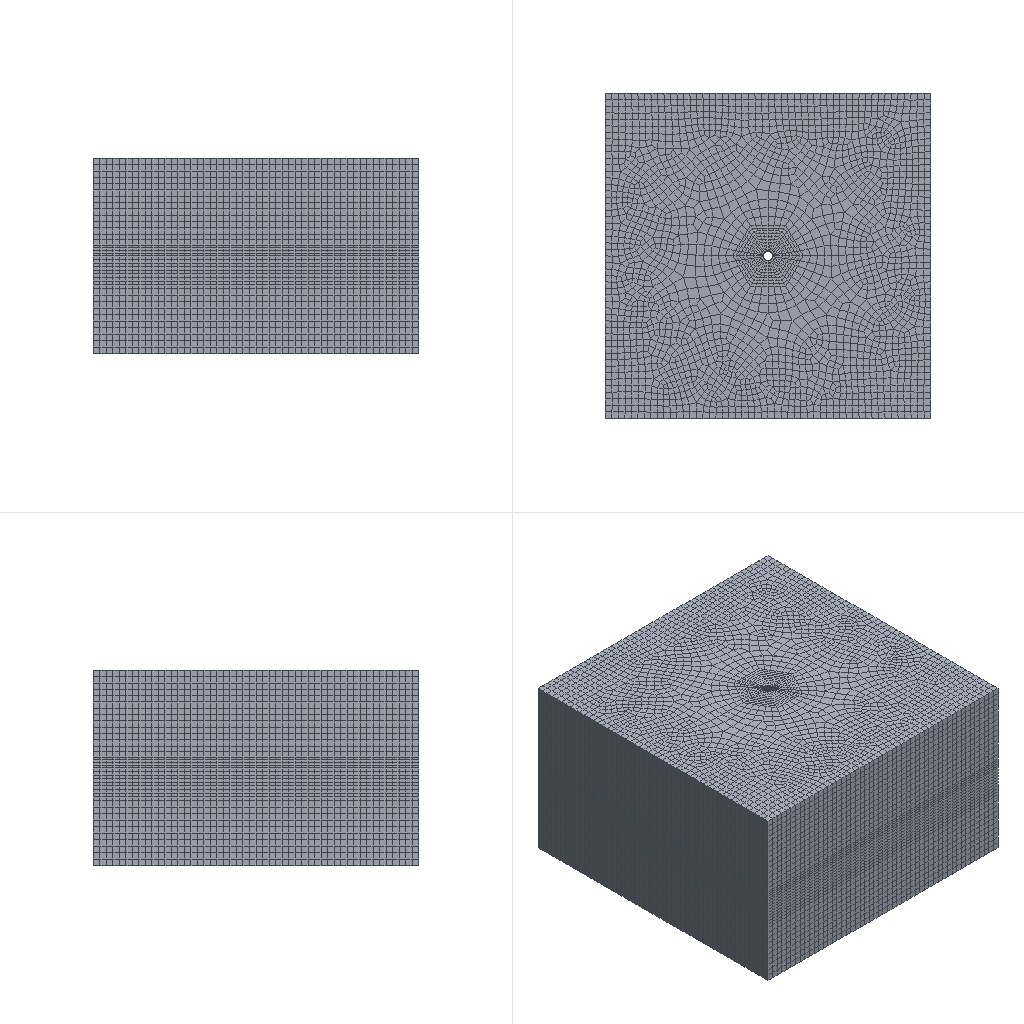Simulation study | abaqus
Set-up summary:
category,name,step,type,value,unit,region
solver,abaqus
solver,version,,,Abaqus/Standard 2020
units,not stated in the deck,,not stated
analysis,deck,,geostatic,geostatic; soils
load_step,Step-1,Step-1,geostatic,nlgeom=False
load_step,Step-2,Step-2,soils,nlgeom=True
contact,interactions,,,general=0 pairs=0 ties=35
load_step,requested,,,2
mesh,nodes,,,104434
mesh,elements,,,96925
element_type,C3D8RP,,solid,96925
load,load commands in deck,,count,3
bc,support commands in deck,,count,6
material,SHUINIHUAN,,in results
material,TAOGUAN,,in results
material,Y,,in results
check,setup vs results,,match,"per instance, exact: element labels, types and connectivity; labels of the nodes the elements use; coordinates of those nodes at SINGLE_PRECISION in 1 of 1 instance(s)"
Abaqus input file, long lists of numbers shortened:
*Heading
** Job name: Job-1 Model name: Model-1-Copy
** Generated by: Abaqus/CAE 2020
*Preprint, echo=NO, model=NO, history=NO, contact=NO
**
** PARTS
**
*Part, name=new
*Node
      1, 0.04, 0.06928,           1.
      2, 0.04, 0.06928,    1.171
** (104432 more lines like these left out)
*Element, type=C3D8RP
 1,   487,     1,   493,  5500,  5503,   502,  5534, 36186
 2,  5501,   490,   489,  5499, 36187,  5518,  5519, 36185
** (96923 more lines like these left out)
*Nset, nset=Set-40
     1,     2,     3,     4,     5,    11,    14,    15,    18,    19,    22,    23,    26,    27,    30,    46
    47,    48,    49,    50,    51,    52,    53,    54,    55,    56,    65,    66,    67,    68,    69,    70
** (166 more lines like these left out)
*Elset, elset=Set-40
   964,   965,   966,   967,   968,   969,   970,   971,   972,   973,   974,   975,   976,   977,   978,   979
   980,   981,   982,   983,   984,   985,   986,   987,   988,   989,   990,   991,   992,   993,   994,   995
** (79 more lines like these left out)
*Nset, nset=Set-41
     1,     2,     3,     4,     5,    11,    14,    15,    18,    19,    22,    23,    26,    27,    30,    46
    47,    48,    49,    50,    51,    52,    53,    54,    55,    56,    65,    66,    67,    68,    69,    70
** (166 more lines like these left out)
*Elset, elset=Set-41
   964,   965,   966,   967,   968,   969,   970,   971,   972,   973,   974,   975,   976,   977,   978,   979
   980,   981,   982,   983,   984,   985,   986,   987,   988,   989,   990,   991,   992,   993,   994,   995
** (79 more lines like these left out)
*Nset, nset=Set-42, generate
      1,  104434,       1
*Elset, elset=Set-42, generate
     1,  96925,      1
** Section: Section-2
*Solid Section, elset=Set-42, material=shuinihuan
,
*End Part
**
**
** ASSEMBLY
**
*Assembly, name=Assembly
**
*Instance, name=new-1, part=new
*End Instance
**
*Nset, nset=Set-5, instance=new-1
     9,    10,    31,    49,    55,    58,    62,    63,    68,    69,    75,    76,    77,    83,    84,    88
    90,    91,    97,   102,   104,   105,   108,   133,   144,   166,   178,   179,   182,   189,   190,   191
** (6 more lines like these left out)
*Elset, elset=Set-5, instance=new-1
   729,  1269,  1413,  1415,  1488,  1517,  1518,  1523,  1542,  1753,  1834,  2053,  2133,  2138,  2152,  2478
  2479,  2480,  2481,  3579,  3580,  3584,  3587,  3711,  4756,  5511,  6123,  6259,  6263,  6270,  6273,  6971
** (3 more lines like these left out)
*Nset, nset=Set-6, instance=new-1
     9,    10,    31,    49,    55,    58,    62,    63,    68,    69,    75,    76,    77,    83,    84,    88
    90,    91,    97,   102,   104,   105,   108,   133,   144,   166,   178,   179,   182,   189,   190,   191
** (6 more lines like these left out)
*Elset, elset=Set-6, instance=new-1
   729,  1269,  1413,  1415,  1488,  1517,  1518,  1523,  1542,  1753,  1834,  2053,  2133,  2138,  2152,  2478
  2479,  2480,  2481,  3579,  3580,  3584,  3587,  3711,  4756,  5511,  6123,  6259,  6263,  6270,  6273,  6971
** (3 more lines like these left out)
*Nset, nset=Set-7, instance=new-1
   426,   427,   428,   429,   430,   431,   432,   433,   434,   435,   436,   437,   438,   439,   440,   441
   447,   448,   449,   450,   456,   457,   458,   459,   479,   480,   481,   482,   483,   484,   485,   486
** (241 more lines like these left out)
*Elset, elset=Set-7, instance=new-1
 15663, 15666, 15667, 15668, 15690, 15691, 15692, 15694, 15695, 15696, 15746, 15747, 15749, 15772, 15774, 15804
 15805, 15808, 15810, 15822, 15834, 15835, 15836, 15845, 15850, 15852, 15859, 15860, 15861, 15863, 15865, 15866
** (230 more lines like these left out)
*Nset, nset=Set-8, instance=new-1
   426,   427,   428,   429,   430,   431,   432,   433,   434,   435,   436,   437,   438,   439,   440,   441
   447,   448,   449,   450,   456,   457,   458,   459,   479,   480,   481,   482,   483,   484,   485,   486
** (241 more lines like these left out)
*Elset, elset=Set-8, instance=new-1
 15663, 15669, 15713, 15714, 15716, 15717, 15718, 15720, 15731, 15787, 15788, 15790, 15792, 15811, 15823, 15824
 15826, 15827, 15828, 15840, 15841, 15847, 15848, 15850, 15920, 15922, 15924, 15925, 15927, 15929, 15930, 15932
** (230 more lines like these left out)
*Nset, nset=Set-9, instance=new-1
    27,    28,    29,    30,    44,    45,    51,    53,    54,    56,    57,    59,    60,    61,    85,    87
    89,    93,    96,    98,    99,   100,   101,   121,   122,   123,   124,   139,   140,   141,   142,   152
** (342 more lines like these left out)
*Elset, elset=Set-9, instance=new-1
   694,   695,   696,   697,   698,   699,   700,   701,   702,   703,   704,   705,   706,   707,   708,   709
   710,   711,   712,   713,   714,   715,   716,   717,   718,   719,   720,   955,   956,   957,   958,   959
** (335 more lines like these left out)
*Nset, nset=Set-10, instance=new-1
   426,   427,   428,   429,   430,   431,   432,   433,   434,   435,   436,   437,   438,   439,   440,   441
   447,   448,   449,   450,   456,   457,   458,   459,   479,   480,   481,   482,   483,   484,   485,   486
** (473 more lines like these left out)
*Elset, elset=Set-10, instance=new-1
 15663, 15666, 15667, 15668, 15669, 15690, 15691, 15692, 15694, 15695, 15696, 15713, 15714, 15716, 15717, 15718
 15720, 15731, 15746, 15747, 15749, 15772, 15774, 15787, 15788, 15790, 15792, 15804, 15805, 15808, 15810, 15811
** (452 more lines like these left out)
*Nset, nset=Set-11, instance=new-1
     3,     4,     5,     8,     9,    10,    13,    14,    17,    18,    21,    22,    25,    26,    29,    30
    46,    47,    48,    49,    50,    52,    53,    54,    55,    56,    58,    59,    62,    63,    64,    65
** (244 more lines like these left out)
*Elset, elset=Set-11, instance=new-1
     3,     5,     6,     8,    11,    13,    14,    16,    19,    21,    22,    24,    27,    29,    30,    32
    35,    37,    38,    40,    43,    45,    46,    48,    51,    53,    54,    56,    59,    61,    62,    64
** (339 more lines like these left out)
*Nset, nset=Set-12, instance=new-1, generate
      1,  104434,       1
*Elset, elset=Set-12, instance=new-1, generate
     1,  96925,      1
*Nset, nset=Set-13, instance=new-1, generate
      1,  104434,       1
*Elset, elset=Set-13, instance=new-1, generate
     1,  96925,      1
*Nset, nset=Set-14, instance=new-1, generate
      1,  104434,       1
*Elset, elset=Set-14, instance=new-1, generate
     1,  96925,      1
*Elset, elset=__T0_new-1_M_S2, internal, instance=new-1, generate
 739,  747,    1
*Surface, type=ELEMENT, name=_T0_new-1_M, internal
__T0_new-1_M_S2, S2
*Elset, elset=__T0_new-1_S_S3, internal, instance=new-1
 71304,
*Surface, type=ELEMENT, name=_T0_new-1_S, internal
__T0_new-1_S_S3, S3
*Tie, name=_T0_new-1, adjust=no
_T0_new-1_S, _T0_new-1_M
*Elset, elset=__T1_new-1_M_S2, internal, instance=new-1, generate
 1298,  1325,     1
*Surface, type=ELEMENT, name=_T1_new-1_M, internal
__T1_new-1_M_S2, S2
*Elset, elset=__T1_new-1_S_S3, internal, instance=new-1, generate
 77799,  92954,   2165
*Surface, type=ELEMENT, name=_T1_new-1_S, internal
__T1_new-1_S_S3, S3
*Tie, name=_T1_new-1, adjust=no
_T1_new-1_S, _T1_new-1_M
*Elset, elset=__T2_new-1_M_S4, internal, instance=new-1
 42011, 44176
*Elset, elset=__T2_new-1_M_S6, internal, instance=new-1
 42010, 44175
*Elset, elset=__T2_new-1_M_S5, internal, instance=new-1
 42009, 44174
*Surface, type=ELEMENT, name=_T2_new-1_M, internal
__T2_new-1_M_S4, S4
__T2_new-1_M_S6, S6
__T2_new-1_M_S5, S5
*Elset, elset=__T2_new-1_S_S2, internal, instance=new-1
 1511,
*Surface, type=ELEMENT, name=_T2_new-1_S, internal
__T2_new-1_S_S2, S2
*Tie, name=_T2_new-1, adjust=no
_T2_new-1_S, _T2_new-1_M
*Nset, nset=_T2_new-1_SN, instance=new-1
 6563,
*Surface, type=NODE, name=_T2_new-1_SN, internal
_T2_new-1_SN
*Tie, name=_T2_new-1-Nodes, adjust=no
_T2_new-1_SN, _T2_new-1_M
*Elset, elset=__T3_new-1_M_S2, internal, instance=new-1, generate
 1801,  1824,     1
*Surface, type=ELEMENT, name=_T3_new-1_M, internal
__T3_new-1_M_S2, S2
*Elset, elset=__T3_new-1_S_S6, internal, instance=new-1, generate
 77808,  92963,   2165
*Surface, type=ELEMENT, name=_T3_new-1_S, internal
__T3_new-1_S_S6, S6
*Tie, name=_T3_new-1, adjust=no
_T3_new-1_S, _T3_new-1_M
*Elset, elset=__T4_new-1_M_S4, internal, instance=new-1, generate
 69149,  73479,   2165
*Elset, elset=__T4_new-1_M_S6, internal, instance=new-1, generate
 69148,  73478,   2165
*Elset, elset=__T4_new-1_M_S5, internal, instance=new-1, generate
 69147,  73477,   2165
*Surface, type=ELEMENT, name=_T4_new-1_M, internal
__T4_new-1_M_S4, S4
__T4_new-1_M_S6, S6
__T4_new-1_M_S5, S5
*Elset, elset=__T4_new-1_S_S2, internal, instance=new-1
 1849,
*Surface, type=ELEMENT, name=_T4_new-1_S, internal
__T4_new-1_S_S2, S2
*Tie, name=_T4_new-1, adjust=no
_T4_new-1_S, _T4_new-1_M
*Nset, nset=_T4_new-1_SN, instance=new-1
 6759,
*Surface, type=NODE, name=_T4_new-1_SN, internal
_T4_new-1_SN
*Tie, name=_T4_new-1-Nodes, adjust=no
_T4_new-1_SN, _T4_new-1_M
*Elset, elset=__T5_new-1_M_S2, internal, instance=new-1, generate
 2099,  2121,     1
*Surface, type=ELEMENT, name=_T5_new-1_M, internal
__T5_new-1_M_S2, S2
*Elset, elset=__T5_new-1_S_S6, internal, instance=new-1, generate
 18195,  37680,   2165
*Surface, type=ELEMENT, name=_T5_new-1_S, internal
__T5_new-1_S_S6, S6
*Tie, name=_T5_new-1, adjust=no
_T5_new-1_S, _T5_new-1_M
*Elset, elset=__T6_new-1_M_S2, internal, instance=new-1, generate
 2162,  2170,     1
*Surface, type=ELEMENT, name=_T6_new-1_M, internal
__T6_new-1_M_S2, S2
*Elset, elset=__T6_new-1_S_S6, internal, instance=new-1
 57506,
*Surface, type=ELEMENT, name=_T6_new-1_S, internal
__T6_new-1_S_S6, S6
*Tie, name=_T6_new-1, adjust=no
_T6_new-1_S, _T6_new-1_M
*Elset, elset=__T7_new-1_M_S5, internal, instance=new-1, generate
 47995,  54490,   2165
*Elset, elset=__T7_new-1_M_S6, internal, instance=new-1, generate
 46369,  52864,   2165
*Elset, elset=__T7_new-1_M_S4, internal, instance=new-1, generate
 46368,  52863,   2165
*Surface, type=ELEMENT, name=_T7_new-1_M, internal
__T7_new-1_M_S5, S5
__T7_new-1_M_S6, S6
__T7_new-1_M_S4, S4
*Elset, elset=__T7_new-1_S_S2, internal, instance=new-1
 2501,
*Surface, type=ELEMENT, name=_T7_new-1_S, internal
__T7_new-1_S_S2, S2
*Tie, name=_T7_new-1, adjust=no
_T7_new-1_S, _T7_new-1_M
*Nset, nset=_T7_new-1_SN, instance=new-1
 7236, 7237, 7241, 7243, 7244
*Surface, type=NODE, name=_T7_new-1_SN, internal
_T7_new-1_SN
*Tie, name=_T7_new-1-Nodes, adjust=no
_T7_new-1_SN, _T7_new-1_M
*Elset, elset=__T8_new-1_M_S2, internal, instance=new-1, generate
 3721,  3729,     1
*Surface, type=ELEMENT, name=_T8_new-1_M, internal
__T8_new-1_M_S2, S2
*Elset, elset=__T8_new-1_S_S3, internal, instance=new-1
 65862,
*Surface, type=ELEMENT, name=_T8_new-1_S, internal
__T8_new-1_S_S3, S3
*Tie, name=_T8_new-1, adjust=no
_T8_new-1_S, _T8_new-1_M
*Elset, elset=__T9_new-1_M_S2, internal, instance=new-1, generate
 4774,  4782,     1
*Surface, type=ELEMENT, name=_T9_new-1_M, internal
__T9_new-1_M_S2, S2
*Elset, elset=__T9_new-1_S_S3, internal, instance=new-1
 59133,
*Surface, type=ELEMENT, name=_T9_new-1_S, internal
__T9_new-1_S_S3, S3
*Tie, name=_T9_new-1, adjust=no
_T9_new-1_S, _T9_new-1_M
*Elset, elset=__T10_new-1_M_S2, internal, instance=new-1, generate
 5521,  5529,     1
*Surface, type=ELEMENT, name=_T10_new-1_M, internal
__T10_new-1_M_S2, S2
*Elset, elset=__T10_new-1_S_S6, internal, instance=new-1
 57230,
*Surface, type=ELEMENT, name=_T10_new-1_S, internal
__T10_new-1_S_S6, S6
*Tie, name=_T10_new-1, adjust=no
_T10_new-1_S, _T10_new-1_M
*Elset, elset=__T11_new-1_M_S2, internal, instance=new-1, generate
 6133,  6141,     1
*Surface, type=ELEMENT, name=_T11_new-1_M, internal
__T11_new-1_M_S2, S2
*Elset, elset=__T11_new-1_S_S6, internal, instance=new-1
 63959,
*Surface, type=ELEMENT, name=_T11_new-1_S, internal
__T11_new-1_S_S6, S6
*Tie, name=_T11_new-1, adjust=no
_T11_new-1_S, _T11_new-1_M
*Elset, elset=__T12_new-1_M_S5, internal, instance=new-1
 62027, 62398, 64192, 64563, 66357, 66728
*Elset, elset=__T12_new-1_M_S3, internal, instance=new-1, generate
 63739,  68069,   2165
*Surface, type=ELEMENT, name=_T12_new-1_M, internal
__T12_new-1_M_S5, S5
__T12_new-1_M_S3, S3
*Elset, elset=__T12_new-1_S_S2, internal, instance=new-1
 6982,
*Surface, type=ELEMENT, name=_T12_new-1_S, internal
__T12_new-1_S_S2, S2
*Tie, name=_T12_new-1, adjust=no
_T12_new-1_S, _T12_new-1_M
*Nset, nset=_T12_new-1_SN, instance=new-1
 9599,
*Surface, type=NODE, name=_T12_new-1_SN, internal
_T12_new-1_SN
*Tie, name=_T12_new-1-Nodes, adjust=no
_T12_new-1_SN, _T12_new-1_M
*Elset, elset=__T13_new-1_M_S2, internal, instance=new-1, generate
 7541,  7549,     1
*Surface, type=ELEMENT, name=_T13_new-1_M, internal
__T13_new-1_M_S2, S2
*Elset, elset=__T13_new-1_S_S5, internal, instance=new-1
 71299,
*Surface, type=ELEMENT, name=_T13_new-1_S, internal
__T13_new-1_S_S5, S5
*Tie, name=_T13_new-1, adjust=no
_T13_new-1_S, _T13_new-1_M
*Elset, elset=__T14_new-1_M_S6, internal, instance=new-1
 42019, 42025, 44184, 44190
*Elset, elset=__T14_new-1_M_S4, internal, instance=new-1
 43659, 45824
*Surface, type=ELEMENT, name=_T14_new-1_M, internal
__T14_new-1_M_S6, S6
__T14_new-1_M_S4, S4
*Nset, nset=_T14_new-1_SN, instance=new-1, generate
 9948,  9950,     1
*Surface, type=NODE, name=_T14_new-1_SN, internal
_T14_new-1_SN
*Tie, name=_T14_new-1-Nodes, adjust=no
_T14_new-1_SN, _T14_new-1_M
*Elset, elset=__T15_new-1_M_S2, internal, instance=new-1, generate
 7974,  7998,     1
*Surface, type=ELEMENT, name=_T15_new-1_M, internal
__T15_new-1_M_S2, S2
*Elset, elset=__T15_new-1_S_S6, internal, instance=new-1, generate
 18204,  37689,   2165
*Surface, type=ELEMENT, name=_T15_new-1_S, internal
__T15_new-1_S_S6, S6
*Tie, name=_T15_new-1, adjust=no
_T15_new-1_S, _T15_new-1_M
*Elset, elset=__T16_new-1_M_S2, internal, instance=new-1, generate
 8321,  8345,     1
*Surface, type=ELEMENT, name=_T16_new-1_M, internal
__T16_new-1_M_S2, S2
*Elset, elset=__T16_new-1_S_S6, internal, instance=new-1, generate
 77817,  92972,   2165
*Surface, type=ELEMENT, name=_T16_new-1_S, internal
__T16_new-1_S_S6, S6
*Tie, name=_T16_new-1, adjust=no
_T16_new-1_S, _T16_new-1_M
*Elset, elset=__T17_new-1_M_S2, internal, instance=new-1, generate
 8496,  8504,     1
*Surface, type=ELEMENT, name=_T17_new-1_M, internal
__T17_new-1_M_S2, S2
*Elset, elset=__T17_new-1_S_S6, internal, instance=new-1
 71322,
*Surface, type=ELEMENT, name=_T17_new-1_S, internal
__T17_new-1_S_S6, S6
*Tie, name=_T17_new-1, adjust=no
_T17_new-1_S, _T17_new-1_M
*Elset, elset=__T18_new-1_M_S5, internal, instance=new-1
 42027, 43662, 44192, 45827
*Elset, elset=__T18_new-1_M_S4, internal, instance=new-1
 42026, 44191
*Surface, type=ELEMENT, name=_T18_new-1_M, internal
__T18_new-1_M_S5, S5
__T18_new-1_M_S4, S4
*Elset, elset=__T18_new-1_S_S2, internal, instance=new-1
 9031,
*Surface, type=ELEMENT, name=_T18_new-1_S, internal
__T18_new-1_S_S2, S2
*Tie, name=_T18_new-1, adjust=no
_T18_new-1_S, _T18_new-1_M
*Nset, nset=_T18_new-1_SN, instance=new-1
 10750,
*Surface, type=NODE, name=_T18_new-1_SN, internal
_T18_new-1_SN
*Tie, name=_T18_new-1-Nodes, adjust=no
_T18_new-1_SN, _T18_new-1_M
*Elset, elset=__T19_new-1_M_S2, internal, instance=new-1, generate
 9760,  9769,     1
*Surface, type=ELEMENT, name=_T19_new-1_M, internal
__T19_new-1_M_S2, S2
*Elset, elset=__T19_new-1_S_S5, internal, instance=new-1
 48522, 50687
*Surface, type=ELEMENT, name=_T19_new-1_S, internal
__T19_new-1_S_S5, S5
*Tie, name=_T19_new-1, adjust=no
_T19_new-1_S, _T19_new-1_M
*Elset, elset=__T20_new-1_M_S2, internal, instance=new-1, generate
 9959,  9967,     1
*Surface, type=ELEMENT, name=_T20_new-1_M, internal
__T20_new-1_M_S2, S2
*Elset, elset=__T20_new-1_S_S6, internal, instance=new-1
 71297,
*Surface, type=ELEMENT, name=_T20_new-1_S, internal
__T20_new-1_S_S6, S6
*Tie, name=_T20_new-1, adjust=no
_T20_new-1_S, _T20_new-1_M
*Elset, elset=__T21_new-1_M_S6, internal, instance=new-1
 62023, 62025, 64188, 64190, 66353, 66355
*Elset, elset=__T21_new-1_M_S5, internal, instance=new-1, generate
 62084,  66414,   2165
*Surface, type=ELEMENT, name=_T21_new-1_M, internal
__T21_new-1_M_S6, S6
__T21_new-1_M_S5, S5
*Nset, nset=_T21_new-1_SN, instance=new-1, generate
 11375,  11380,      1
*Surface, type=NODE, name=_T21_new-1_SN, internal
_T21_new-1_SN
*Tie, name=_T21_new-1-Nodes, adjust=no
_T21_new-1_SN, _T21_new-1_M
*Elset, elset=__T22_new-1_M_S2, internal, instance=new-1, generate
 11345,  11353,      1
*Surface, type=ELEMENT, name=_T22_new-1_M, internal
__T22_new-1_M_S2, S2
*Elset, elset=__T22_new-1_S_S6, internal, instance=new-1
 71301,
*Surface, type=ELEMENT, name=_T22_new-1_S, internal
__T22_new-1_S_S6, S6
*Tie, name=_T22_new-1, adjust=no
_T22_new-1_S, _T22_new-1_M
*Elset, elset=__T23_new-1_M_S2, internal, instance=new-1, generate
 11884,  11910,      1
*Surface, type=ELEMENT, name=_T23_new-1_M, internal
__T23_new-1_M_S2, S2
*Elset, elset=__T23_new-1_S_S6, internal, instance=new-1, generate
 77796,  92951,   2165
*Surface, type=ELEMENT, name=_T23_new-1_S, internal
__T23_new-1_S_S6, S6
*Tie, name=_T23_new-1, adjust=no
_T23_new-1_S, _T23_new-1_M
*Elset, elset=__T24_new-1_M_S6, internal, instance=new-1
 41980, 42199, 44145, 44364
*Elset, elset=__T24_new-1_M_S5, internal, instance=new-1
 41660, 43825
*Surface, type=ELEMENT, name=_T24_new-1_M, internal
__T24_new-1_M_S6, S6
__T24_new-1_M_S5, S5
*Elset, elset=__T24_new-1_S_S2, internal, instance=new-1
 12840, 12841, 12846, 12847, 12849, 12854, 12855
*Surface, type=ELEMENT, name=_T24_new-1_S, internal
__T24_new-1_S_S2, S2
*Tie, name=_T24_new-1, adjust=no
_T24_new-1_S, _T24_new-1_M
*Elset, elset=__T25_new-1_M_S2, internal, instance=new-1, generate
 13904,  13913,      1
*Surface, type=ELEMENT, name=_T25_new-1_M, internal
__T25_new-1_M_S2, S2
*Elset, elset=__T25_new-1_S_S6, internal, instance=new-1
 48694, 50859
*Surface, type=ELEMENT, name=_T25_new-1_S, internal
__T25_new-1_S_S6, S6
*Tie, name=_T25_new-1, adjust=no
_T25_new-1_S, _T25_new-1_M
*Elset, elset=__T26_new-1_M_S5, internal, instance=new-1, generate
 46384,  52879,   2165
*Elset, elset=__T26_new-1_M_S3, internal, instance=new-1, generate
 46366,  52861,   2165
*Elset, elset=__T26_new-1_M_S6, internal, instance=new-1, generate
 46311,  52806,   2165
*Surface, type=ELEMENT, name=_T26_new-1_M, internal
__T26_new-1_M_S5, S5
__T26_new-1_M_S3, S3
__T26_new-1_M_S6, S6
*Elset, elset=__T26_new-1_S_S2, internal, instance=new-1
 15345, 15355
*Surface, type=ELEMENT, name=_T26_new-1_S, internal
__T26_new-1_S_S2, S2
*Tie, name=_T26_new-1, adjust=no
_T26_new-1_S, _T26_new-1_M
*Nset, nset=_T26_new-1_SN, instance=new-1
 13364, 13371, 13372
*Surface, type=NODE, name=_T26_new-1_SN, internal
_T26_new-1_SN
*Tie, name=_T26_new-1-Nodes, adjust=no
_T26_new-1_SN, _T26_new-1_M
*Elset, elset=__T27_new-1_M_S5, internal, instance=new-1, generate
 55356,  59686,   2165
*Elset, elset=__T27_new-1_M_S3, internal, instance=new-1, generate
 55338,  59668,   2165
*Elset, elset=__T27_new-1_M_S6, internal, instance=new-1, generate
 55283,  59613,   2165
*Surface, type=ELEMENT, name=_T27_new-1_M, internal
__T27_new-1_M_S5, S5
__T27_new-1_M_S3, S3
__T27_new-1_M_S6, S6
*Elset, elset=__T27_new-1_S_S2, internal, instance=new-1
 15511,
*Surface, type=ELEMENT, name=_T27_new-1_S, internal
__T27_new-1_S_S2, S2
*Tie, name=_T27_new-1, adjust=no
_T27_new-1_S, _T27_new-1_M
*Nset, nset=_T27_new-1_SN, instance=new-1
 13415, 13417
*Surface, type=NODE, name=_T27_new-1_SN, internal
_T27_new-1_SN
*Tie, name=_T27_new-1-Nodes, adjust=no
_T27_new-1_SN, _T27_new-1_M
*Nset, nset=Set-10_PP_, internal, instance=new-1
   426,   427,   428,   429,   430,   431,   432,   433,   434,   435,   436,   437,   438,   439,   440,   441
   447,   448,   449,   450,   456,   457,   458,   459,   479,   480,   481,   482,   483,   484,   485,   486
** (473 more lines like these left out)
*Nset, nset=Set-11_PP_, internal, instance=new-1
     3,     4,     5,     8,     9,    10,    13,    14,    17,    18,    21,    22,    25,    26,    29,    30
    46,    47,    48,    49,    50,    52,    53,    54,    55,    56,    58,    59,    62,    63,    64,    65
** (244 more lines like these left out)
*End Assembly
*Amplitude, name=Amp-1
             0.,              0.,              1.,              1.
**
** MATERIALS
**
*Material, name=Y
*Elastic
 9e+09, 0.25
*Permeability, specific=9800.
 7e-07, 0.1
*Material, name=shuinihuan
*Elastic
 9e+09, 0.25
*Permeability, specific=9800.
 7e-07, 0.1
*Material, name=taoguan
*Elastic
 2.11e+11, 0.21
**
** PREDEFINED FIELDS
**
** Name: Predefined Field-1   Type: Stress
*Initial Conditions, type=STRESS
Set-12, -3.5e+07, -3e+07, -4e+07, 0., 0., 0.
** Name: Predefined Field-2   Type: Void ratio
*Initial Conditions, TYPE=RATIO
Set-13, 0.12
** Name: Predefined Field-3   Type: Saturation
*Initial Conditions, type=SATURATION
Set-14, 1.
** ----------------------------------------------------------------
**
** STEP: Step-1
**
*Step, name=Step-1, nlgeom=NO, unsymm=YES
*Geostatic
**
** BOUNDARY CONDITIONS
**
** Name: BC-1 Type: 位移/转角
*Boundary
Set-7, 2, 2
** Name: BC-2 Type: 位移/转角
*Boundary
Set-8, 1, 1
** Name: BC-3 Type: 位移/转角
*Boundary
Set-9, 3, 3
** Name: BC-4 Type: 孔隙压力
*Boundary
Set-10_PP_, 8, 8, 2.5e+07
** Name: BC-5 Type: 孔隙压力
*Boundary
Set-11_PP_, 8, 8, 2e+07
**
** OUTPUT REQUESTS
**
*Restart, write, frequency=0
**
** FIELD OUTPUT: F-Output-1
**
*Output, field
*Node Output
CF, POR, RF, U, V
*Element Output, directions=YES
E, FLUVR, FLVEL, LE, MISES, MISESMAX, MISESONLY, NE, PE, PEEQ, PEEQMAX, PEEQT, PEMAG, PRESSONLY, S, SAT
SEQUT, SROCK, SSAVG, VOIDR, YIELDPOT
*Contact Output
CDISP, CSTRESS
**
** HISTORY OUTPUT: H-Output-1
**
*Output, history, variable=PRESELECT
*End Step
** ----------------------------------------------------------------
**
** STEP: Step-2
**
*Step, name=Step-2, nlgeom=YES, inc=1000, unsymm=YES
*Soils, consolidation, end=PERIOD, utol=1e+11, creep=none, stabilize=0.0002, allsdtol=0.05, continue=NO
0.01, 1., 1e-05, 0.1,
**
** BOUNDARY CONDITIONS
**
** Name: BC-5 Type: 孔隙压力
*Boundary, amplitude=Amp-1
Set-11_PP_, 8, 8, 1e+08
**
** OUTPUT REQUESTS
**
*Restart, write, frequency=0
**
** FIELD OUTPUT: F-Output-1
**
*Output, field
*Node Output
CF, POR, RF, U, V
*Element Output, directions=YES
E, FLUVR, FLVEL, LE, MISES, MISESMAX, MISESONLY, NE, PE, PEEQ, PEEQMAX, PEEQT, PEMAG, PRESSONLY, S, SAT
SEQUT, SROCK, SSAVG, VOIDR, YIELDPOT
*Contact Output
CDISP, CSTRESS
**
** HISTORY OUTPUT: H-Output-1
**
*Output, history, variable=PRESELECT
*End Step
Results summary:
result,step,,completed,increments=1 time=1.0/1.0
result,step,,completed,increments=16 time=1.0/1.0
result,analysis,,,"soils, consolidation"
result,last_loadstep,,,2
result,analysis steps,,count,2
result,primary field,,,"U, POR"
result,reaction total,,FX,-0.9844,model units
result,reaction total,,FY,1.875,model units
result,reaction total,,FZ,0.1035,model units